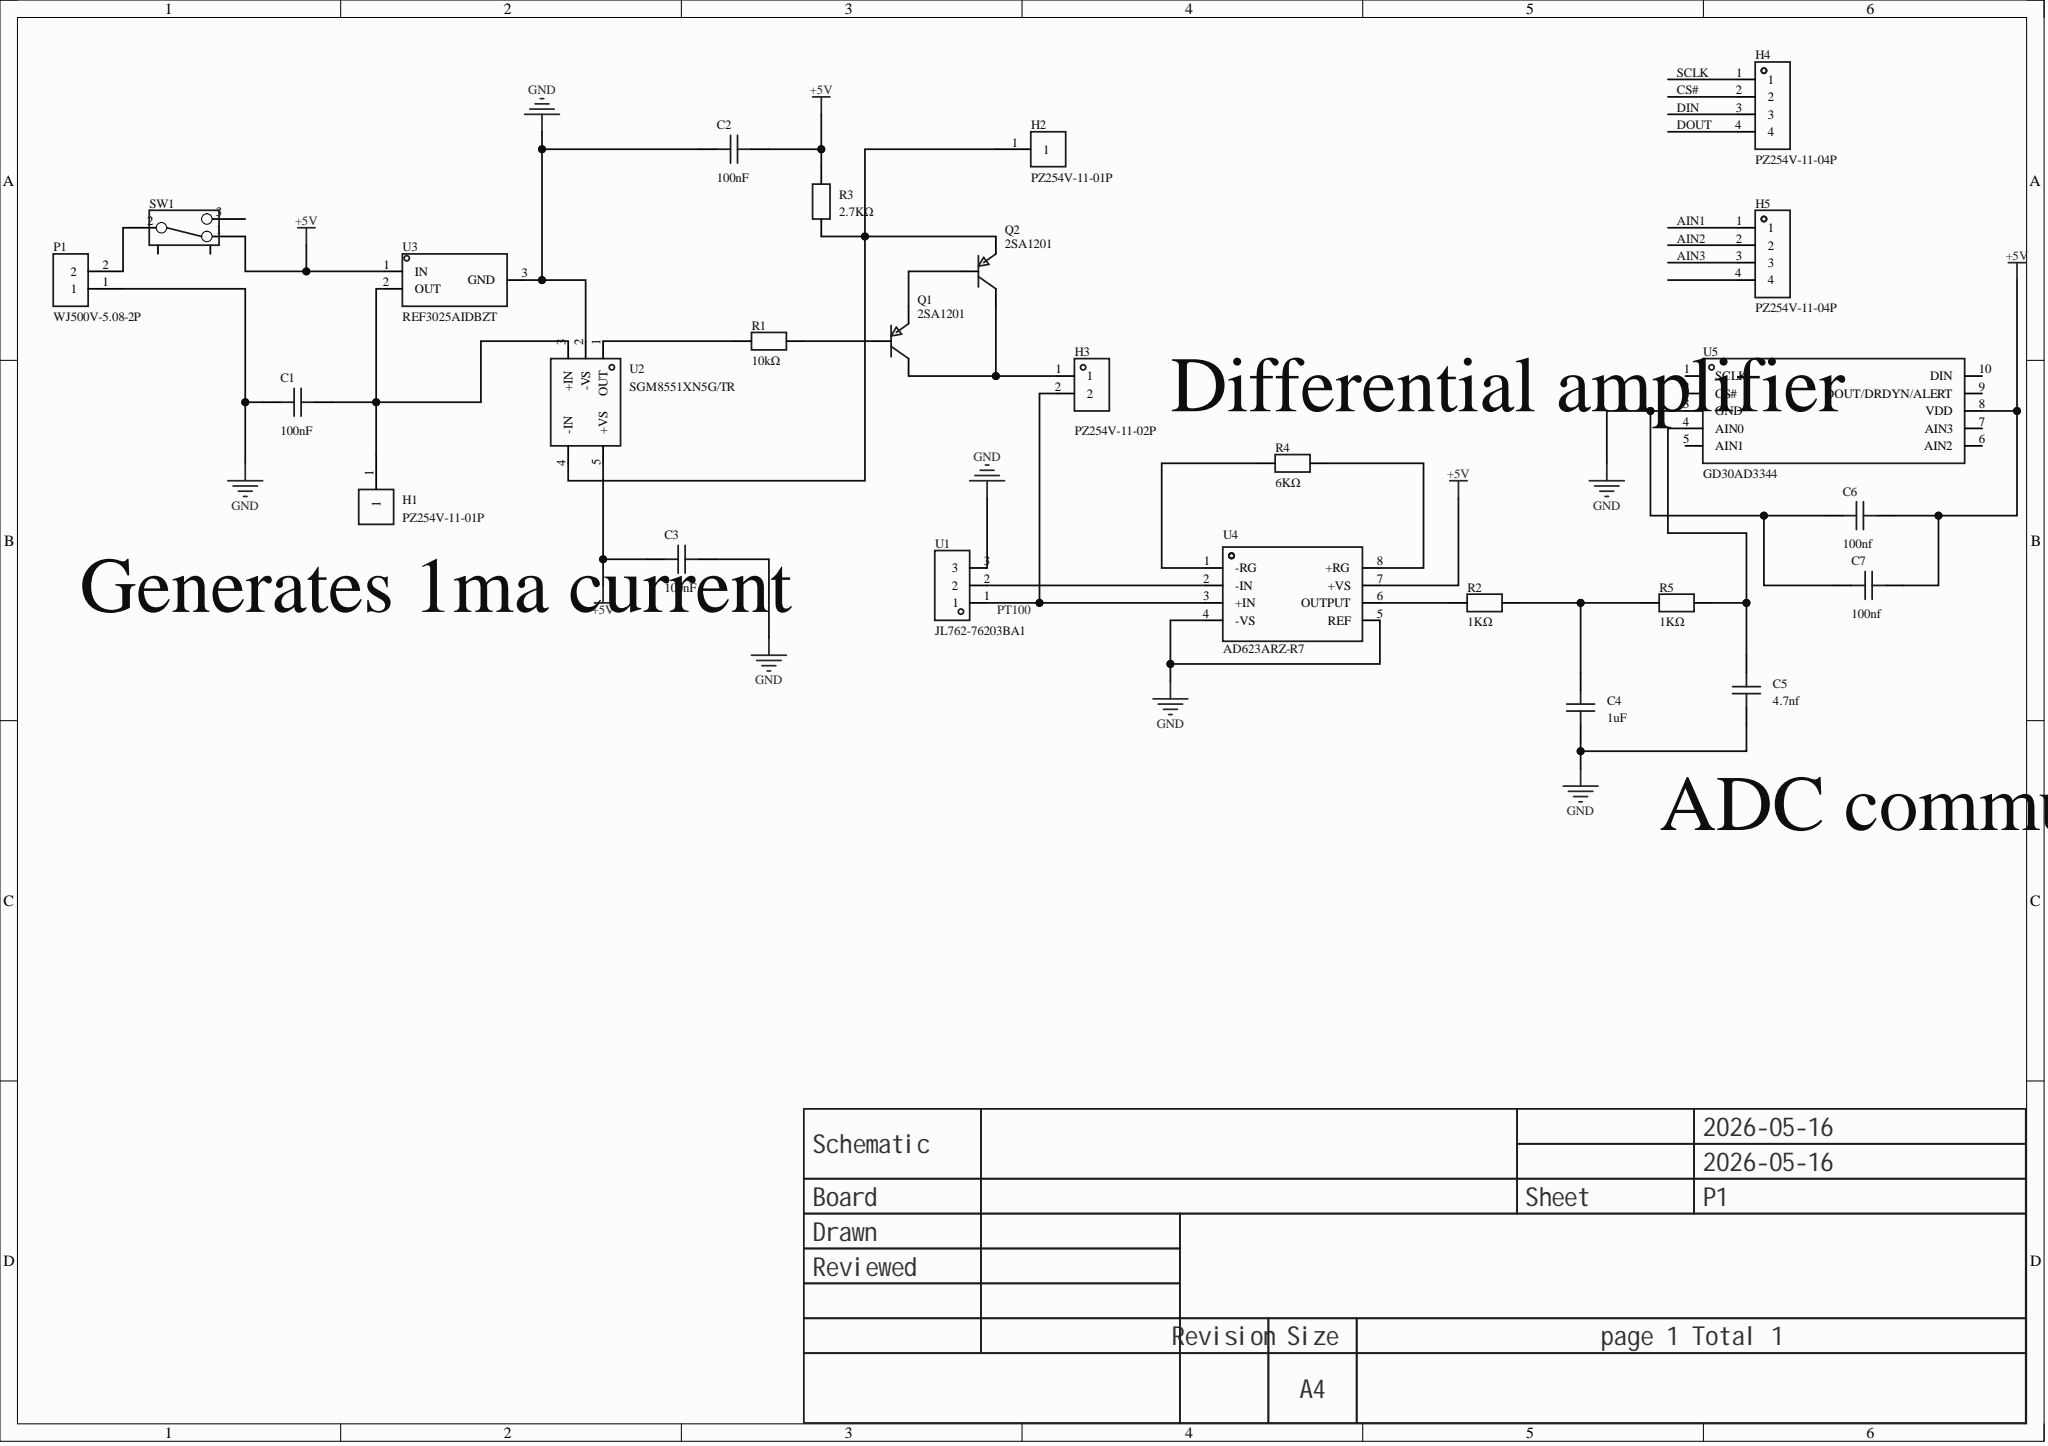Circuit board | Altium Designer | 26 parts | 16 nets
Bill of materials:
Comment,Description,Designator,Footprint,LibRef,Quantity
"100nF","Capacitance:100nF;Tolerance:±10%;Rated voltage:50V;Temperature coefficient:X7R;","C1, C2, C3, C6, C7","CAP-SMD_L2.0-W1.25","FCC0805B104K500DT","5"
"1uF","Capacitance:100nF;Tolerance:±10%;Rated voltage:50V;Temperature coefficient:X7R;","C4","CAP-SMD_L2.0-W1.25","FCC0805B104K500DT","1"
"4.7nf","Capacitance:100nF;Tolerance:±10%;Rated voltage:50V;Temperature coefficient:X7R;","C5","CAP-SMD_L2.0-W1.25","FCC0805B104K500DT","1"
"PZ254V-11-01P","","H1, H2","HDR-TH_1P-P2.54-V-M","PZ254V-11-01P","2"
"PZ254V-11-02P","","H3","HDR-TH_2P-P2.54-V-M","PZ254V-11-02P","1"
"PZ254V-11-04P","","H4, H5","HDR-TH_4P-P2.54-V-M","PZ254V-11-04P","2"
"WJ500V-5.08-2P","","P1","CONN-TH_2P-P5.00_WJ500V-5.08-2P","WJ500V-5.08-2P","1"
"2SA1201","Transistor type:PNP;Collector current (Ic):800mA;Collector-emitter breakdown voltage (Vceo):120V;Power dissipation (Pd):500mW;DC current gain (hFE):240@100mA,5V;","Q1, Q2","SOT-89-3_L4.5-W2.5-P1.50-LS4.2-BR","2SA1201","2"
"10kΩ","Resistor type:Thick film resistor;Resistance:10kΩ;Tolerance:±5%;Power:125mW;Working voltage:150V;Temperature coefficient:±100ppm/?;","R1","R0805","FRC0805J103TS","1"
"1KΩ","Resistor type:Thin film resistor;Resistance:500mΩ;Tolerance:±1%;Power:1W;Temperature coefficient:±100ppm/?;","R2, R5","R1206","HoJLRH1206-1W-500mR-1%","2"
"2.7KΩ","Resistor type:Thin film resistor;Resistance:500mΩ;Tolerance:±1%;Power:1W;Temperature coefficient:±100ppm/?;","R3","R1206","HoJLRH1206-1W-500mR-1%","1"
"6KΩ","Resistor type:Thin film resistor;Resistance:500mΩ;Tolerance:±1%;Power:1W;Temperature coefficient:±100ppm/?;","R4","R1206","HoJLRH1206-1W-500mR-1%","1"
"","","SW1","拨动开关","拨动开关_正","1"
"JL762-76203BA1","","U1","CONN-TH_JL762-76203BA1","JL762-76203BA1","1"
"SGM8551XN5G/TR","Amplifier count:-;","U2","SOT-23-5_L3.0-W1.7-P0.95-LS2.8-BL","SGM8551XN5G/TR","1"
"REF3025AIDBZT","Output type:Fixed;Operating voltage:2.55V~5.5V;Output voltage:2.5V;Output current:25mA;Accuracy:±0.2%;","U3","SOT-23-3_L3.0-W1.7-P0.95-LS2.9-BR","REF3025AIDBZT","1"
"AD623ARZ-R7","Amplifier count:Single;Common-mode rejection ratio (CMRR):80dB;Input bias current (Ib):25nA;Input offset voltage (Vos):200uV;Gain bandwidth product (GBP):-;Slew rate (SR):0.3V/us;Rail to rail:Rail-to-rail output;","U4","SOIC-8_L5.0-W4.0-P1.27-LS6.0-BL","AD623ARZ-R7","1"
"GD30AD3344","","U5","MSOP-10_L3.0-W3.0-P0.50-LS5.0-BL","GD30AD3344","1"
Netlist (Protel format):
[
C1
CAP-SMD_L2.0-W1.25
100nF



]
[
C2
CAP-SMD_L2.0-W1.25
100nF



]
[
C3
CAP-SMD_L2.0-W1.25
100nF



]
[
C4
CAP-SMD_L2.0-W1.25
1uF



]
[
C5
CAP-SMD_L2.0-W1.25
4.7nf



]
[
C6
CAP-SMD_L2.0-W1.25
100nf



]
[
C7
CAP-SMD_L2.0-W1.25
100nf



]
[
H1
HDR-TH_1P-P2.54-V-M
PZ254V-11-01P



]
[
H2
HDR-TH_1P-P2.54-V-M
PZ254V-11-01P



]
[
H3
HDR-TH_2P-P2.54-V-M
PZ254V-11-02P



]
[
H4
HDR-TH_4P-P2.54-V-M
PZ254V-11-04P



]
[
H5
HDR-TH_4P-P2.54-V-M
PZ254V-11-04P



]
[
P1
CONN-TH_2P-P5.00_WJ500V-5.08-2P
WJ500V-5.08-2P



]
[
Q1
SOT-89-3_L4.5-W2.5-P1.50-LS4.2-BR
2SA1201



]
[
Q2
SOT-89-3_L4.5-W2.5-P1.50-LS4.2-BR
2SA1201



]
[
R1
R0805
10kΩ



]
[
R2
R1206
1KΩ



]
[
R3
R1206
2.7KΩ



]
[
R4
R1206
6KΩ



]
[
R5
R1206
1KΩ



]
[
SW1
拨动开关




]
[
U1
CONN-TH_JL762-76203BA1
JL762-76203BA1



]
[
U2
SOT-23-5_L3.0-W1.7-P0.95-LS2.8-BL
SGM8551XN5G/TR



]
[
U3
SOT-23-3_L3.0-W1.7-P0.95-LS2.9-BR
REF3025AIDBZT



]
[
U4
SOIC-8_L5.0-W4.0-P1.27-LS6.0-BL
AD623ARZ-R7



]
[
U5
MSOP-10_L3.0-W3.0-P0.50-LS5.0-BL
GD30AD3344



]
(
PT100
H3-2
U1-1
U4-3
)
(
NetU1_2
U1-2
U4-2
)
(
NetR4_2
R4-2
U4-1
)
(
NetR4_1
R4-1
U4-8
)
(
NetR2_1
R2-1
U4-6
)
(
NetR1_1
R1-1
U2-1
)
(
NetQ1_3
Q1-3
Q2-1
)
(
NetQ1_1
Q1-1
R1-2
)
(
NetP1_2
P1-2
SW1-2
)
(
NetH3_1
H3-1
Q1-2
Q2-2
)
(
NetH2_1
H2-1
Q2-3
R3-1
U2-4
)
(
NetC5_2
C5-2
R5-2
U5-4
)
(
NetC4_2
C4-2
R2-2
R5-1
)
(
NetC1_2
C1-2
H1-1
U2-3
U3-2
)
(
GND
C1-1
C2-1
C3-2
C4-1
C5-1
C6-2
C7-2
P1-1
U1-3
U2-2
U3-3
U4-4
U4-5
U5-3
)
(
+5V
C2-2
C3-1
C6-1
C7-1
R3-2
SW1-1
U2-5
U3-1
U4-7
U5-8
)